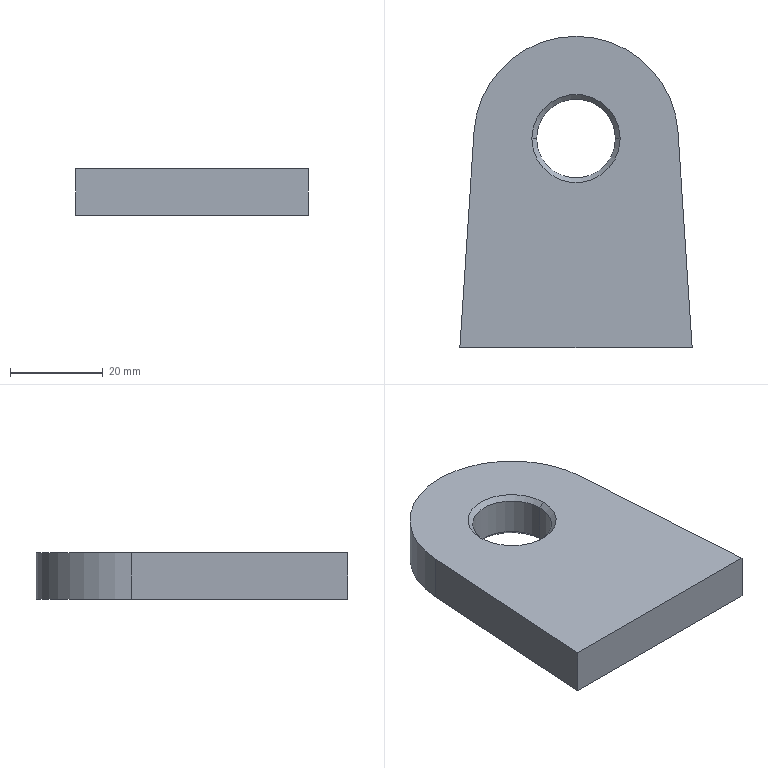Part | SolidWorks | features Chamfer 1, Extrusion 1 | 1 solid | 12 faces | box 50 x 67 x 10 mm | volume 26449 mm3 | plane 5 | cone 4 | cylinder 3 | commonest cylinder face diameters 17 x2 44 x1
STEP:
#1=CARTESIAN_POINT('',(16.5,45.,9.));
#2=VERTEX_POINT('',#1);
#3=CARTESIAN_POINT('',(33.5,45.,9.));
#4=VERTEX_POINT('',#3);
#5=CARTESIAN_POINT('',(25.,45.,9.));
#6=DIRECTION('',(0.,0.,1.));
#7=DIRECTION('',(1.,0.,0.));
#8=AXIS2_PLACEMENT_3D('',#5,#6,#7);
#9=CIRCLE('',#8,8.5);
#10=EDGE_CURVE('',#2,#4,#9,.T.);
#11=ORIENTED_EDGE('',*,*,#10,.F.);
#12=CARTESIAN_POINT('',(15.5,45.,10.));
#13=VERTEX_POINT('',#12);
#14=CARTESIAN_POINT('',(16.5,45.,9.));
#15=DIRECTION('',(-0.7071,0.,0.7071));
#16=VECTOR('',#15,1000.);
#17=LINE('',#14,#16);
#18=EDGE_CURVE('',#2,#13,#17,.T.);
#19=ORIENTED_EDGE('',*,*,#18,.T.);
#20=CARTESIAN_POINT('',(34.5,45.,10.));
#21=VERTEX_POINT('',#20);
#22=CARTESIAN_POINT('',(25.,45.,10.));
#23=DIRECTION('',(0.,0.,-1.));
#24=DIRECTION('',(1.,0.,0.));
#25=AXIS2_PLACEMENT_3D('',#22,#23,#24);
#26=CIRCLE('',#25,9.5);
#27=EDGE_CURVE('',#21,#13,#26,.T.);
#28=ORIENTED_EDGE('',*,*,#27,.F.);
#29=CARTESIAN_POINT('',(33.5,45.,9.));
#30=DIRECTION('',(0.7071,0.,0.7071));
#31=VECTOR('',#30,1000.);
#32=LINE('',#29,#31);
#33=EDGE_CURVE('',#4,#21,#32,.T.);
#34=ORIENTED_EDGE('',*,*,#33,.F.);
#35=EDGE_LOOP('',(#11,#19,#28,#34));
#36=FACE_OUTER_BOUND('',#35,.T.);
#37=CARTESIAN_POINT('',(25.,45.,9.));
#38=DIRECTION('',(0.,0.,1.));
#39=DIRECTION('',(1.,0.,0.));
#40=AXIS2_PLACEMENT_3D('',#37,#38,#39);
#41=CONICAL_SURFACE('',#40,8.5,0.7854);
#42=ADVANCED_FACE('',(#36),#41,.F.);
#43=CARTESIAN_POINT('',(33.5,45.,1.));
#44=VERTEX_POINT('',#43);
#45=CARTESIAN_POINT('',(16.5,45.,1.));
#46=VERTEX_POINT('',#45);
#47=CARTESIAN_POINT('',(25.,45.,1.));
#48=DIRECTION('',(0.,0.,-1.));
#49=DIRECTION('',(1.,0.,0.));
#50=AXIS2_PLACEMENT_3D('',#47,#48,#49);
#51=CIRCLE('',#50,8.5);
#52=EDGE_CURVE('',#44,#46,#51,.T.);
#53=ORIENTED_EDGE('',*,*,#52,.F.);
#54=CARTESIAN_POINT('',(34.5,45.,0.));
#55=VERTEX_POINT('',#54);
#56=CARTESIAN_POINT('',(34.5,45.,0.));
#57=DIRECTION('',(0.7071,0.,-0.7071));
#58=VECTOR('',#57,1000.);
#59=LINE('',#56,#58);
#60=EDGE_CURVE('',#44,#55,#59,.T.);
#61=ORIENTED_EDGE('',*,*,#60,.T.);
#62=CARTESIAN_POINT('',(15.5,45.,0.));
#63=VERTEX_POINT('',#62);
#64=CARTESIAN_POINT('',(25.,45.,0.));
#65=DIRECTION('',(0.,0.,1.));
#66=DIRECTION('',(1.,0.,0.));
#67=AXIS2_PLACEMENT_3D('',#64,#65,#66);
#68=CIRCLE('',#67,9.5);
#69=EDGE_CURVE('',#63,#55,#68,.T.);
#70=ORIENTED_EDGE('',*,*,#69,.F.);
#71=CARTESIAN_POINT('',(15.5,45.,0.));
#72=DIRECTION('',(-0.7071,0.,-0.7071));
#73=VECTOR('',#72,1000.);
#74=LINE('',#71,#73);
#75=EDGE_CURVE('',#46,#63,#74,.T.);
#76=ORIENTED_EDGE('',*,*,#75,.F.);
#77=EDGE_LOOP('',(#53,#61,#70,#76));
#78=FACE_OUTER_BOUND('',#77,.T.);
#79=CARTESIAN_POINT('',(25.,45.,0.));
#80=DIRECTION('',(0.,0.,-1.));
#81=DIRECTION('',(-1.,0.,0.));
#82=AXIS2_PLACEMENT_3D('',#79,#80,#81);
#83=CONICAL_SURFACE('',#82,9.5,0.7854);
#84=ADVANCED_FACE('',(#78),#83,.F.);
#85=ORIENTED_EDGE('',*,*,#10,.T.);
#86=CARTESIAN_POINT('',(33.5,45.,10.));
#87=DIRECTION('',(0.,0.,-1.));
#88=VECTOR('',#87,1000.);
#89=LINE('',#86,#88);
#90=EDGE_CURVE('',#4,#44,#89,.T.);
#91=ORIENTED_EDGE('',*,*,#90,.T.);
#92=ORIENTED_EDGE('',*,*,#52,.T.);
#93=CARTESIAN_POINT('',(16.5,45.,10.));
#94=DIRECTION('',(0.,0.,-1.));
#95=VECTOR('',#94,1000.);
#96=LINE('',#93,#95);
#97=EDGE_CURVE('',#2,#46,#96,.T.);
#98=ORIENTED_EDGE('',*,*,#97,.F.);
#99=EDGE_LOOP('',(#85,#91,#92,#98));
#100=FACE_OUTER_BOUND('',#99,.T.);
#101=CARTESIAN_POINT('',(25.,45.,10.));
#102=DIRECTION('',(0.,0.,-1.));
#103=DIRECTION('',(-1.,0.,0.));
#104=AXIS2_PLACEMENT_3D('',#101,#102,#103);
#105=CYLINDRICAL_SURFACE('',#104,8.5);
#106=ADVANCED_FACE('',(#100),#105,.F.);
#107=ORIENTED_EDGE('',*,*,#27,.T.);
#108=CARTESIAN_POINT('',(25.,45.,10.));
#109=DIRECTION('',(0.,0.,-1.));
#110=DIRECTION('',(1.,0.,0.));
#111=AXIS2_PLACEMENT_3D('',#108,#109,#110);
#112=CIRCLE('',#111,9.5);
#113=EDGE_CURVE('',#13,#21,#112,.T.);
#114=ORIENTED_EDGE('',*,*,#113,.T.);
#115=EDGE_LOOP('',(#107,#114));
#116=FACE_BOUND('',#115,.T.);
#117=CARTESIAN_POINT('',(3.047,46.44,10.));
#118=VERTEX_POINT('',#117);
#119=CARTESIAN_POINT('',(0.,0.,10.));
#120=VERTEX_POINT('',#119);
#121=CARTESIAN_POINT('',(0.,0.,10.));
#122=DIRECTION('',(-0.06547,-0.9979,0.));
#123=VECTOR('',#122,1000.);
#124=LINE('',#121,#123);
#125=EDGE_CURVE('',#118,#120,#124,.T.);
#126=ORIENTED_EDGE('',*,*,#125,.T.);
#127=CARTESIAN_POINT('',(50.,0.,10.));
#128=VERTEX_POINT('',#127);
#129=CARTESIAN_POINT('',(0.,0.,10.));
#130=DIRECTION('',(1.,0.,0.));
#131=VECTOR('',#130,1000.);
#132=LINE('',#129,#131);
#133=EDGE_CURVE('',#120,#128,#132,.T.);
#134=ORIENTED_EDGE('',*,*,#133,.T.);
#135=CARTESIAN_POINT('',(46.953,46.44,10.));
#136=VERTEX_POINT('',#135);
#137=CARTESIAN_POINT('',(50.,0.,10.));
#138=DIRECTION('',(-0.06547,0.9979,0.));
#139=VECTOR('',#138,1000.);
#140=LINE('',#137,#139);
#141=EDGE_CURVE('',#128,#136,#140,.T.);
#142=ORIENTED_EDGE('',*,*,#141,.T.);
#143=CARTESIAN_POINT('',(25.,45.,10.));
#144=DIRECTION('',(0.,0.,1.));
#145=DIRECTION('',(1.,0.,0.));
#146=AXIS2_PLACEMENT_3D('',#143,#144,#145);
#147=CIRCLE('',#146,22.);
#148=EDGE_CURVE('',#136,#118,#147,.T.);
#149=ORIENTED_EDGE('',*,*,#148,.T.);
#150=EDGE_LOOP('',(#126,#134,#142,#149));
#151=FACE_OUTER_BOUND('',#150,.T.);
#152=CARTESIAN_POINT('',(25.,45.,10.));
#153=DIRECTION('',(0.,0.,1.));
#154=DIRECTION('',(1.,0.,0.));
#155=AXIS2_PLACEMENT_3D('',#152,#153,#154);
#156=PLANE('',#155);
#157=ADVANCED_FACE('',(#116,#151),#156,.T.);
#158=ORIENTED_EDGE('',*,*,#69,.T.);
#159=CARTESIAN_POINT('',(25.,45.,0.));
#160=DIRECTION('',(0.,0.,1.));
#161=DIRECTION('',(1.,0.,0.));
#162=AXIS2_PLACEMENT_3D('',#159,#160,#161);
#163=CIRCLE('',#162,9.5);
#164=EDGE_CURVE('',#55,#63,#163,.T.);
#165=ORIENTED_EDGE('',*,*,#164,.T.);
#166=EDGE_LOOP('',(#158,#165));
#167=FACE_BOUND('',#166,.T.);
#168=CARTESIAN_POINT('',(3.047,46.44,0.));
#169=VERTEX_POINT('',#168);
#170=CARTESIAN_POINT('',(0.,0.,0.));
#171=VERTEX_POINT('',#170);
#172=CARTESIAN_POINT('',(0.,0.,0.));
#173=DIRECTION('',(-0.06547,-0.9979,0.));
#174=VECTOR('',#173,1000.);
#175=LINE('',#172,#174);
#176=EDGE_CURVE('',#169,#171,#175,.T.);
#177=ORIENTED_EDGE('',*,*,#176,.F.);
#178=CARTESIAN_POINT('',(46.953,46.44,0.));
#179=VERTEX_POINT('',#178);
#180=CARTESIAN_POINT('',(25.,45.,0.));
#181=DIRECTION('',(0.,0.,1.));
#182=DIRECTION('',(1.,0.,0.));
#183=AXIS2_PLACEMENT_3D('',#180,#181,#182);
#184=CIRCLE('',#183,22.);
#185=EDGE_CURVE('',#179,#169,#184,.T.);
#186=ORIENTED_EDGE('',*,*,#185,.F.);
#187=CARTESIAN_POINT('',(50.,0.,0.));
#188=VERTEX_POINT('',#187);
#189=CARTESIAN_POINT('',(50.,0.,0.));
#190=DIRECTION('',(-0.06547,0.9979,0.));
#191=VECTOR('',#190,1000.);
#192=LINE('',#189,#191);
#193=EDGE_CURVE('',#188,#179,#192,.T.);
#194=ORIENTED_EDGE('',*,*,#193,.F.);
#195=CARTESIAN_POINT('',(0.,0.,0.));
#196=DIRECTION('',(1.,0.,0.));
#197=VECTOR('',#196,1000.);
#198=LINE('',#195,#197);
#199=EDGE_CURVE('',#171,#188,#198,.T.);
#200=ORIENTED_EDGE('',*,*,#199,.F.);
#201=EDGE_LOOP('',(#177,#186,#194,#200));
#202=FACE_OUTER_BOUND('',#201,.T.);
#203=CARTESIAN_POINT('',(25.,45.,0.));
#204=DIRECTION('',(0.,0.,1.));
#205=DIRECTION('',(1.,0.,0.));
#206=AXIS2_PLACEMENT_3D('',#203,#204,#205);
#207=PLANE('',#206);
#208=ADVANCED_FACE('',(#167,#202),#207,.F.);
#209=ORIENTED_EDGE('',*,*,#176,.T.);
#210=CARTESIAN_POINT('',(0.,0.,10.));
#211=DIRECTION('',(0.,0.,-1.));
#212=VECTOR('',#211,1000.);
#213=LINE('',#210,#212);
#214=EDGE_CURVE('',#120,#171,#213,.T.);
#215=ORIENTED_EDGE('',*,*,#214,.F.);
#216=ORIENTED_EDGE('',*,*,#125,.F.);
#217=CARTESIAN_POINT('',(3.047,46.44,10.));
#218=DIRECTION('',(0.,0.,-1.));
#219=VECTOR('',#218,1000.);
#220=LINE('',#217,#219);
#221=EDGE_CURVE('',#118,#169,#220,.T.);
#222=ORIENTED_EDGE('',*,*,#221,.T.);
#223=EDGE_LOOP('',(#209,#215,#216,#222));
#224=FACE_OUTER_BOUND('',#223,.T.);
#225=CARTESIAN_POINT('',(0.,0.,10.));
#226=DIRECTION('',(0.9979,-0.06547,0.));
#227=DIRECTION('',(0.06547,0.9979,0.));
#228=AXIS2_PLACEMENT_3D('',#225,#226,#227);
#229=PLANE('',#228);
#230=ADVANCED_FACE('',(#224),#229,.F.);
#231=ORIENTED_EDGE('',*,*,#199,.T.);
#232=CARTESIAN_POINT('',(50.,0.,10.));
#233=DIRECTION('',(0.,0.,-1.));
#234=VECTOR('',#233,1000.);
#235=LINE('',#232,#234);
#236=EDGE_CURVE('',#128,#188,#235,.T.);
#237=ORIENTED_EDGE('',*,*,#236,.F.);
#238=ORIENTED_EDGE('',*,*,#133,.F.);
#239=ORIENTED_EDGE('',*,*,#214,.T.);
#240=EDGE_LOOP('',(#231,#237,#238,#239));
#241=FACE_OUTER_BOUND('',#240,.T.);
#242=CARTESIAN_POINT('',(0.,0.,10.));
#243=DIRECTION('',(0.,1.,0.));
#244=DIRECTION('',(0.,0.,1.));
#245=AXIS2_PLACEMENT_3D('',#242,#243,#244);
#246=PLANE('',#245);
#247=ADVANCED_FACE('',(#241),#246,.F.);
#248=ORIENTED_EDGE('',*,*,#193,.T.);
#249=CARTESIAN_POINT('',(46.953,46.44,10.));
#250=DIRECTION('',(0.,0.,-1.));
#251=VECTOR('',#250,1000.);
#252=LINE('',#249,#251);
#253=EDGE_CURVE('',#136,#179,#252,.T.);
#254=ORIENTED_EDGE('',*,*,#253,.F.);
#255=ORIENTED_EDGE('',*,*,#141,.F.);
#256=ORIENTED_EDGE('',*,*,#236,.T.);
#257=EDGE_LOOP('',(#248,#254,#255,#256));
#258=FACE_OUTER_BOUND('',#257,.T.);
#259=CARTESIAN_POINT('',(50.,0.,10.));
#260=DIRECTION('',(-0.9979,-0.06547,0.));
#261=DIRECTION('',(0.06547,-0.9979,0.));
#262=AXIS2_PLACEMENT_3D('',#259,#260,#261);
#263=PLANE('',#262);
#264=ADVANCED_FACE('',(#258),#263,.F.);
#265=ORIENTED_EDGE('',*,*,#185,.T.);
#266=ORIENTED_EDGE('',*,*,#221,.F.);
#267=ORIENTED_EDGE('',*,*,#148,.F.);
#268=ORIENTED_EDGE('',*,*,#253,.T.);
#269=EDGE_LOOP('',(#265,#266,#267,#268));
#270=FACE_OUTER_BOUND('',#269,.T.);
#271=CARTESIAN_POINT('',(25.,45.,10.));
#272=DIRECTION('',(0.,0.,-1.));
#273=DIRECTION('',(-1.,0.,0.));
#274=AXIS2_PLACEMENT_3D('',#271,#272,#273);
#275=CYLINDRICAL_SURFACE('',#274,22.);
#276=ADVANCED_FACE('',(#270),#275,.T.);
#277=ORIENTED_EDGE('',*,*,#90,.F.);
#278=CARTESIAN_POINT('',(25.,45.,9.));
#279=DIRECTION('',(0.,0.,1.));
#280=DIRECTION('',(1.,0.,0.));
#281=AXIS2_PLACEMENT_3D('',#278,#279,#280);
#282=CIRCLE('',#281,8.5);
#283=EDGE_CURVE('',#4,#2,#282,.T.);
#284=ORIENTED_EDGE('',*,*,#283,.T.);
#285=ORIENTED_EDGE('',*,*,#97,.T.);
#286=CARTESIAN_POINT('',(25.,45.,1.));
#287=DIRECTION('',(0.,0.,-1.));
#288=DIRECTION('',(1.,0.,0.));
#289=AXIS2_PLACEMENT_3D('',#286,#287,#288);
#290=CIRCLE('',#289,8.5);
#291=EDGE_CURVE('',#46,#44,#290,.T.);
#292=ORIENTED_EDGE('',*,*,#291,.T.);
#293=EDGE_LOOP('',(#277,#284,#285,#292));
#294=FACE_OUTER_BOUND('',#293,.T.);
#295=CARTESIAN_POINT('',(25.,45.,10.));
#296=DIRECTION('',(0.,0.,-1.));
#297=DIRECTION('',(-1.,0.,0.));
#298=AXIS2_PLACEMENT_3D('',#295,#296,#297);
#299=CYLINDRICAL_SURFACE('',#298,8.5);
#300=ADVANCED_FACE('',(#294),#299,.F.);
#301=ORIENTED_EDGE('',*,*,#60,.F.);
#302=ORIENTED_EDGE('',*,*,#291,.F.);
#303=ORIENTED_EDGE('',*,*,#75,.T.);
#304=ORIENTED_EDGE('',*,*,#164,.F.);
#305=EDGE_LOOP('',(#301,#302,#303,#304));
#306=FACE_OUTER_BOUND('',#305,.T.);
#307=CARTESIAN_POINT('',(25.,45.,0.));
#308=DIRECTION('',(0.,0.,-1.));
#309=DIRECTION('',(-1.,0.,0.));
#310=AXIS2_PLACEMENT_3D('',#307,#308,#309);
#311=CONICAL_SURFACE('',#310,9.5,0.7854);
#312=ADVANCED_FACE('',(#306),#311,.F.);
#313=ORIENTED_EDGE('',*,*,#18,.F.);
#314=ORIENTED_EDGE('',*,*,#283,.F.);
#315=ORIENTED_EDGE('',*,*,#33,.T.);
#316=ORIENTED_EDGE('',*,*,#113,.F.);
#317=EDGE_LOOP('',(#313,#314,#315,#316));
#318=FACE_OUTER_BOUND('',#317,.T.);
#319=CARTESIAN_POINT('',(25.,45.,9.));
#320=DIRECTION('',(0.,0.,1.));
#321=DIRECTION('',(1.,0.,0.));
#322=AXIS2_PLACEMENT_3D('',#319,#320,#321);
#323=CONICAL_SURFACE('',#322,8.5,0.7854);
#324=ADVANCED_FACE('',(#318),#323,.F.);
#325=CLOSED_SHELL('',(#42,#84,#106,#157,#208,#230,#247,#264,#276,#300,#312,#324));
#326=MANIFOLD_SOLID_BREP('',#325);
#327=CARTESIAN_POINT('',(0.,0.,0.));
#328=DIRECTION('',(0.,0.,1.));
#329=DIRECTION('',(1.,0.,0.));
#330=AXIS2_PLACEMENT_3D('',#327,#328,#329);
#331=(LENGTH_UNIT()NAMED_UNIT(*)SI_UNIT(.MILLI.,.METRE.));
#332=UNCERTAINTY_MEASURE_WITH_UNIT(LENGTH_MEASURE(0.00001),#331,'','');
#333=(NAMED_UNIT(*)PLANE_ANGLE_UNIT()SI_UNIT($,.RADIAN.));
#334=(NAMED_UNIT(*)SI_UNIT($,.STERADIAN.)SOLID_ANGLE_UNIT());
#335=(GEOMETRIC_REPRESENTATION_CONTEXT(3)GLOBAL_UNCERTAINTY_ASSIGNED_CONTEXT((#332))GLOBAL_UNIT_ASSIGNED_CONTEXT((#331,#333,#334))REPRESENTATION_CONTEXT('',''));
#336=ADVANCED_BREP_SHAPE_REPRESENTATION('',(#326,#330),#335);